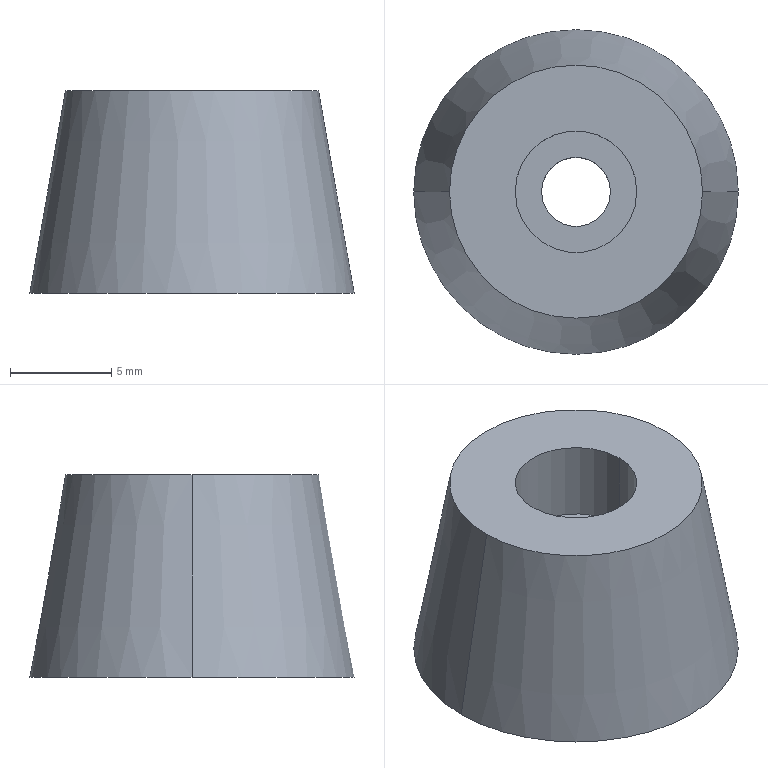Part | SolidWorks | features Extrusion 1, HoleWzd 1 | 1 solid | 9 faces | box 16 x 16 x 10 mm | volume 1432 mm3 | cylinder 4 | plane 3 | cone 2 | commonest cylinder face diameters 3.4 x2 6 x2
STEP:
#1=CARTESIAN_POINT('',(-3.,0.,6.));
#2=VERTEX_POINT('',#1);
#3=CARTESIAN_POINT('',(3.,0.,6.));
#4=VERTEX_POINT('',#3);
#5=CARTESIAN_POINT('',(0.,0.,6.));
#6=DIRECTION('',(0.,0.,1.));
#7=DIRECTION('',(1.,0.,0.));
#8=AXIS2_PLACEMENT_3D('',#5,#6,#7);
#9=CIRCLE('',#8,3.);
#10=EDGE_CURVE('',#2,#4,#9,.T.);
#11=ORIENTED_EDGE('',*,*,#10,.F.);
#12=CARTESIAN_POINT('',(-3.,0.,10.));
#13=VERTEX_POINT('',#12);
#14=CARTESIAN_POINT('',(-3.,0.,10.));
#15=DIRECTION('',(0.,0.,1.));
#16=VECTOR('',#15,1000.);
#17=LINE('',#14,#16);
#18=EDGE_CURVE('',#2,#13,#17,.T.);
#19=ORIENTED_EDGE('',*,*,#18,.T.);
#20=CARTESIAN_POINT('',(3.,0.,10.));
#21=VERTEX_POINT('',#20);
#22=CARTESIAN_POINT('',(0.,0.,10.));
#23=DIRECTION('',(0.,0.,1.));
#24=DIRECTION('',(1.,0.,0.));
#25=AXIS2_PLACEMENT_3D('',#22,#23,#24);
#26=CIRCLE('',#25,3.);
#27=EDGE_CURVE('',#13,#21,#26,.T.);
#28=ORIENTED_EDGE('',*,*,#27,.T.);
#29=CARTESIAN_POINT('',(3.,0.,10.));
#30=DIRECTION('',(0.,0.,1.));
#31=VECTOR('',#30,1000.);
#32=LINE('',#29,#31);
#33=EDGE_CURVE('',#4,#21,#32,.T.);
#34=ORIENTED_EDGE('',*,*,#33,.F.);
#35=EDGE_LOOP('',(#11,#19,#28,#34));
#36=FACE_OUTER_BOUND('',#35,.T.);
#37=CARTESIAN_POINT('',(0.,0.,10.));
#38=DIRECTION('',(0.,0.,1.));
#39=DIRECTION('',(1.,0.,0.));
#40=AXIS2_PLACEMENT_3D('',#37,#38,#39);
#41=CYLINDRICAL_SURFACE('',#40,3.);
#42=ADVANCED_FACE('',(#36),#41,.F.);
#43=CARTESIAN_POINT('',(-1.7,0.,0.));
#44=VERTEX_POINT('',#43);
#45=CARTESIAN_POINT('',(1.7,0.,0.));
#46=VERTEX_POINT('',#45);
#47=CARTESIAN_POINT('',(0.,0.,0.));
#48=DIRECTION('',(0.,0.,1.));
#49=DIRECTION('',(1.,0.,0.));
#50=AXIS2_PLACEMENT_3D('',#47,#48,#49);
#51=CIRCLE('',#50,1.7);
#52=EDGE_CURVE('',#44,#46,#51,.T.);
#53=ORIENTED_EDGE('',*,*,#52,.F.);
#54=CARTESIAN_POINT('',(-1.7,0.,6.));
#55=VERTEX_POINT('',#54);
#56=CARTESIAN_POINT('',(-1.7,0.,10.));
#57=DIRECTION('',(0.,0.,1.));
#58=VECTOR('',#57,1000.);
#59=LINE('',#56,#58);
#60=EDGE_CURVE('',#44,#55,#59,.T.);
#61=ORIENTED_EDGE('',*,*,#60,.T.);
#62=CARTESIAN_POINT('',(1.7,0.,6.));
#63=VERTEX_POINT('',#62);
#64=CARTESIAN_POINT('',(0.,0.,6.));
#65=DIRECTION('',(0.,0.,1.));
#66=DIRECTION('',(1.,0.,0.));
#67=AXIS2_PLACEMENT_3D('',#64,#65,#66);
#68=CIRCLE('',#67,1.7);
#69=EDGE_CURVE('',#55,#63,#68,.T.);
#70=ORIENTED_EDGE('',*,*,#69,.T.);
#71=CARTESIAN_POINT('',(1.7,0.,10.));
#72=DIRECTION('',(0.,0.,1.));
#73=VECTOR('',#72,1000.);
#74=LINE('',#71,#73);
#75=EDGE_CURVE('',#46,#63,#74,.T.);
#76=ORIENTED_EDGE('',*,*,#75,.F.);
#77=EDGE_LOOP('',(#53,#61,#70,#76));
#78=FACE_OUTER_BOUND('',#77,.T.);
#79=CARTESIAN_POINT('',(0.,0.,10.));
#80=DIRECTION('',(0.,0.,1.));
#81=DIRECTION('',(1.,0.,0.));
#82=AXIS2_PLACEMENT_3D('',#79,#80,#81);
#83=CYLINDRICAL_SURFACE('',#82,1.7);
#84=ADVANCED_FACE('',(#78),#83,.F.);
#85=CARTESIAN_POINT('',(-6.237,0.,10.));
#86=VERTEX_POINT('',#85);
#87=CARTESIAN_POINT('',(6.237,0.,10.));
#88=VERTEX_POINT('',#87);
#89=CARTESIAN_POINT('',(0.,0.,10.));
#90=DIRECTION('',(0.,0.,1.));
#91=DIRECTION('',(1.,0.,0.));
#92=AXIS2_PLACEMENT_3D('',#89,#90,#91);
#93=CIRCLE('',#92,6.237);
#94=EDGE_CURVE('',#86,#88,#93,.T.);
#95=ORIENTED_EDGE('',*,*,#94,.F.);
#96=CARTESIAN_POINT('',(-8.,0.,0.));
#97=VERTEX_POINT('',#96);
#98=CARTESIAN_POINT('',(-8.,0.,0.));
#99=DIRECTION('',(-0.1736,0.,-0.9848));
#100=VECTOR('',#99,1000.);
#101=LINE('',#98,#100);
#102=EDGE_CURVE('',#86,#97,#101,.T.);
#103=ORIENTED_EDGE('',*,*,#102,.T.);
#104=CARTESIAN_POINT('',(8.,0.,0.));
#105=VERTEX_POINT('',#104);
#106=CARTESIAN_POINT('',(0.,0.,0.));
#107=DIRECTION('',(0.,0.,1.));
#108=DIRECTION('',(1.,0.,0.));
#109=AXIS2_PLACEMENT_3D('',#106,#107,#108);
#110=CIRCLE('',#109,8.);
#111=EDGE_CURVE('',#97,#105,#110,.T.);
#112=ORIENTED_EDGE('',*,*,#111,.T.);
#113=CARTESIAN_POINT('',(8.,0.,0.));
#114=DIRECTION('',(0.1736,0.,-0.9848));
#115=VECTOR('',#114,1000.);
#116=LINE('',#113,#115);
#117=EDGE_CURVE('',#88,#105,#116,.T.);
#118=ORIENTED_EDGE('',*,*,#117,.F.);
#119=EDGE_LOOP('',(#95,#103,#112,#118));
#120=FACE_OUTER_BOUND('',#119,.T.);
#121=CARTESIAN_POINT('',(0.,0.,0.));
#122=DIRECTION('',(0.,0.,-1.));
#123=DIRECTION('',(1.,0.,0.));
#124=AXIS2_PLACEMENT_3D('',#121,#122,#123);
#125=CONICAL_SURFACE('',#124,8.,0.1745);
#126=ADVANCED_FACE('',(#120),#125,.T.);
#127=ORIENTED_EDGE('',*,*,#102,.F.);
#128=CARTESIAN_POINT('',(0.,0.,10.));
#129=DIRECTION('',(0.,0.,1.));
#130=DIRECTION('',(1.,0.,0.));
#131=AXIS2_PLACEMENT_3D('',#128,#129,#130);
#132=CIRCLE('',#131,6.237);
#133=EDGE_CURVE('',#88,#86,#132,.T.);
#134=ORIENTED_EDGE('',*,*,#133,.F.);
#135=ORIENTED_EDGE('',*,*,#117,.T.);
#136=CARTESIAN_POINT('',(0.,0.,0.));
#137=DIRECTION('',(0.,0.,1.));
#138=DIRECTION('',(1.,0.,0.));
#139=AXIS2_PLACEMENT_3D('',#136,#137,#138);
#140=CIRCLE('',#139,8.);
#141=EDGE_CURVE('',#105,#97,#140,.T.);
#142=ORIENTED_EDGE('',*,*,#141,.T.);
#143=EDGE_LOOP('',(#127,#134,#135,#142));
#144=FACE_OUTER_BOUND('',#143,.T.);
#145=CARTESIAN_POINT('',(0.,0.,0.));
#146=DIRECTION('',(0.,0.,-1.));
#147=DIRECTION('',(1.,0.,0.));
#148=AXIS2_PLACEMENT_3D('',#145,#146,#147);
#149=CONICAL_SURFACE('',#148,8.,0.1745);
#150=ADVANCED_FACE('',(#144),#149,.T.);
#151=CARTESIAN_POINT('',(0.,0.,10.));
#152=DIRECTION('',(0.,0.,1.));
#153=DIRECTION('',(1.,0.,0.));
#154=AXIS2_PLACEMENT_3D('',#151,#152,#153);
#155=CIRCLE('',#154,3.);
#156=EDGE_CURVE('',#21,#13,#155,.T.);
#157=ORIENTED_EDGE('',*,*,#156,.F.);
#158=ORIENTED_EDGE('',*,*,#27,.F.);
#159=EDGE_LOOP('',(#157,#158));
#160=FACE_BOUND('',#159,.T.);
#161=ORIENTED_EDGE('',*,*,#133,.T.);
#162=ORIENTED_EDGE('',*,*,#94,.T.);
#163=EDGE_LOOP('',(#161,#162));
#164=FACE_OUTER_BOUND('',#163,.T.);
#165=CARTESIAN_POINT('',(0.,0.,10.));
#166=DIRECTION('',(0.,0.,1.));
#167=DIRECTION('',(1.,0.,0.));
#168=AXIS2_PLACEMENT_3D('',#165,#166,#167);
#169=PLANE('',#168);
#170=ADVANCED_FACE('',(#160,#164),#169,.T.);
#171=CARTESIAN_POINT('',(0.,0.,0.));
#172=DIRECTION('',(0.,0.,1.));
#173=DIRECTION('',(1.,0.,0.));
#174=AXIS2_PLACEMENT_3D('',#171,#172,#173);
#175=CIRCLE('',#174,1.7);
#176=EDGE_CURVE('',#46,#44,#175,.T.);
#177=ORIENTED_EDGE('',*,*,#176,.T.);
#178=ORIENTED_EDGE('',*,*,#52,.T.);
#179=EDGE_LOOP('',(#177,#178));
#180=FACE_BOUND('',#179,.T.);
#181=ORIENTED_EDGE('',*,*,#141,.F.);
#182=ORIENTED_EDGE('',*,*,#111,.F.);
#183=EDGE_LOOP('',(#181,#182));
#184=FACE_OUTER_BOUND('',#183,.T.);
#185=CARTESIAN_POINT('',(0.,0.,0.));
#186=DIRECTION('',(0.,0.,1.));
#187=DIRECTION('',(1.,0.,0.));
#188=AXIS2_PLACEMENT_3D('',#185,#186,#187);
#189=PLANE('',#188);
#190=ADVANCED_FACE('',(#180,#184),#189,.F.);
#191=ORIENTED_EDGE('',*,*,#60,.F.);
#192=ORIENTED_EDGE('',*,*,#176,.F.);
#193=ORIENTED_EDGE('',*,*,#75,.T.);
#194=CARTESIAN_POINT('',(0.,0.,6.));
#195=DIRECTION('',(0.,0.,1.));
#196=DIRECTION('',(1.,0.,0.));
#197=AXIS2_PLACEMENT_3D('',#194,#195,#196);
#198=CIRCLE('',#197,1.7);
#199=EDGE_CURVE('',#63,#55,#198,.T.);
#200=ORIENTED_EDGE('',*,*,#199,.T.);
#201=EDGE_LOOP('',(#191,#192,#193,#200));
#202=FACE_OUTER_BOUND('',#201,.T.);
#203=CARTESIAN_POINT('',(0.,0.,10.));
#204=DIRECTION('',(0.,0.,1.));
#205=DIRECTION('',(1.,0.,0.));
#206=AXIS2_PLACEMENT_3D('',#203,#204,#205);
#207=CYLINDRICAL_SURFACE('',#206,1.7);
#208=ADVANCED_FACE('',(#202),#207,.F.);
#209=ORIENTED_EDGE('',*,*,#199,.F.);
#210=ORIENTED_EDGE('',*,*,#69,.F.);
#211=EDGE_LOOP('',(#209,#210));
#212=FACE_BOUND('',#211,.T.);
#213=CARTESIAN_POINT('',(0.,0.,6.));
#214=DIRECTION('',(0.,0.,1.));
#215=DIRECTION('',(1.,0.,0.));
#216=AXIS2_PLACEMENT_3D('',#213,#214,#215);
#217=CIRCLE('',#216,3.);
#218=EDGE_CURVE('',#4,#2,#217,.T.);
#219=ORIENTED_EDGE('',*,*,#218,.T.);
#220=ORIENTED_EDGE('',*,*,#10,.T.);
#221=EDGE_LOOP('',(#219,#220));
#222=FACE_OUTER_BOUND('',#221,.T.);
#223=CARTESIAN_POINT('',(1.7,0.,6.));
#224=DIRECTION('',(0.,0.,-1.));
#225=DIRECTION('',(-1.,0.,0.));
#226=AXIS2_PLACEMENT_3D('',#223,#224,#225);
#227=PLANE('',#226);
#228=ADVANCED_FACE('',(#212,#222),#227,.F.);
#229=ORIENTED_EDGE('',*,*,#18,.F.);
#230=ORIENTED_EDGE('',*,*,#218,.F.);
#231=ORIENTED_EDGE('',*,*,#33,.T.);
#232=ORIENTED_EDGE('',*,*,#156,.T.);
#233=EDGE_LOOP('',(#229,#230,#231,#232));
#234=FACE_OUTER_BOUND('',#233,.T.);
#235=CARTESIAN_POINT('',(0.,0.,10.));
#236=DIRECTION('',(0.,0.,1.));
#237=DIRECTION('',(1.,0.,0.));
#238=AXIS2_PLACEMENT_3D('',#235,#236,#237);
#239=CYLINDRICAL_SURFACE('',#238,3.);
#240=ADVANCED_FACE('',(#234),#239,.F.);
#241=CLOSED_SHELL('',(#42,#84,#126,#150,#170,#190,#208,#228,#240));
#242=MANIFOLD_SOLID_BREP('',#241);
#243=CARTESIAN_POINT('',(0.,0.,0.));
#244=DIRECTION('',(0.,0.,1.));
#245=DIRECTION('',(1.,0.,0.));
#246=AXIS2_PLACEMENT_3D('',#243,#244,#245);
#247=(LENGTH_UNIT()NAMED_UNIT(*)SI_UNIT(.MILLI.,.METRE.));
#248=UNCERTAINTY_MEASURE_WITH_UNIT(LENGTH_MEASURE(0.00001),#247,'','');
#249=(NAMED_UNIT(*)PLANE_ANGLE_UNIT()SI_UNIT($,.RADIAN.));
#250=(NAMED_UNIT(*)SI_UNIT($,.STERADIAN.)SOLID_ANGLE_UNIT());
#251=(GEOMETRIC_REPRESENTATION_CONTEXT(3)GLOBAL_UNCERTAINTY_ASSIGNED_CONTEXT((#248))GLOBAL_UNIT_ASSIGNED_CONTEXT((#247,#249,#250))REPRESENTATION_CONTEXT('',''));
#252=ADVANCED_BREP_SHAPE_REPRESENTATION('',(#242,#246),#251);